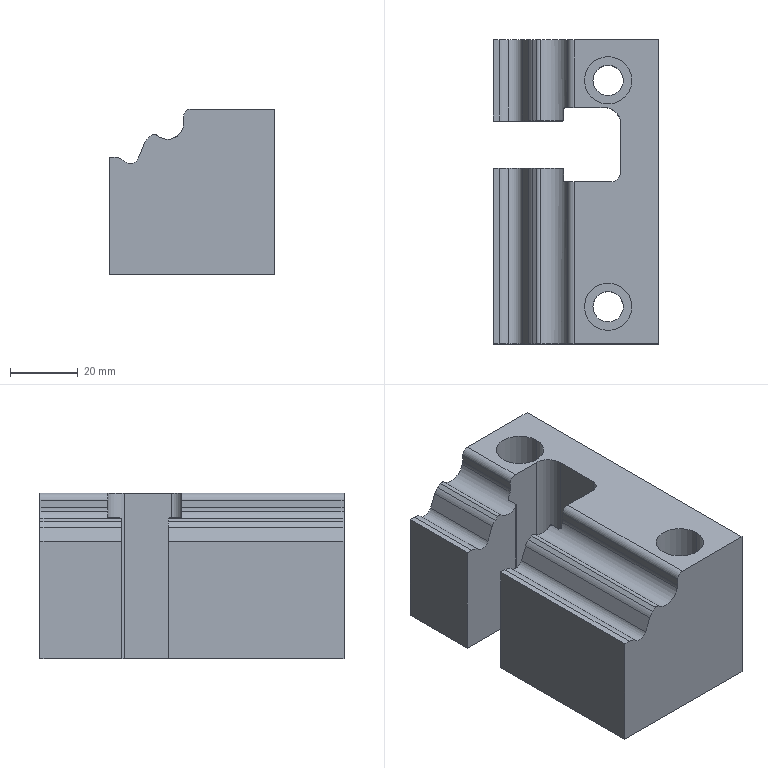Part | 1 solid | 52 faces | box 49 x 90 x 48.948 mm | volume 156743 mm3 | cylinder 28 | plane 24 | commonest cylinder face diameters 1 x4 9 x4 9.5 x4 14 x4 2 x2 4 x2